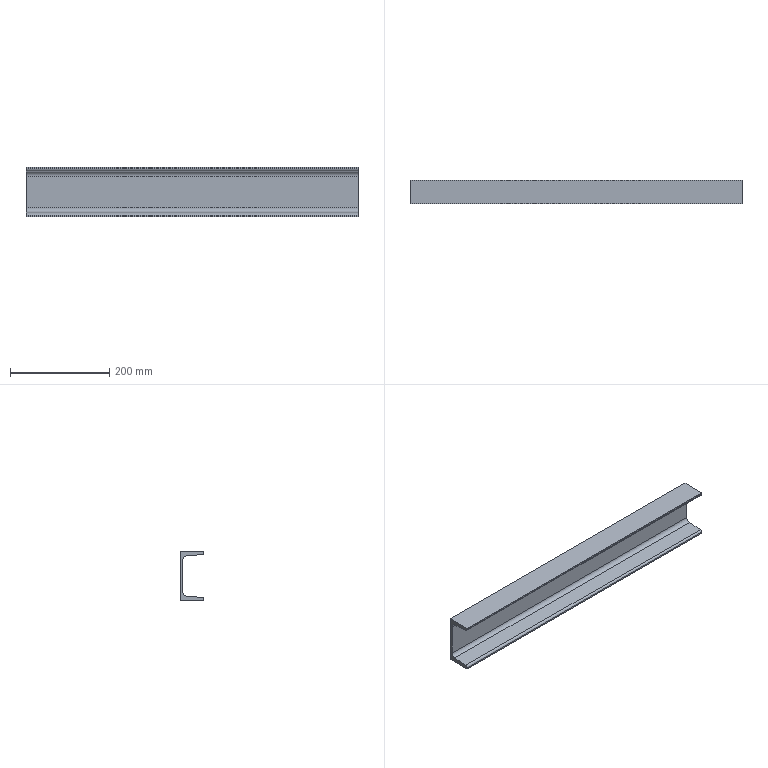Part | STEP file | 06-Channel 100x48_default<machining> | 1 solid | 14 faces | box 670 x 48 x 100 mm | volume 842936 mm3 | plane 10 | cylinder 4 | commonest cylinder face diameters 8.5 x2 17 x2
STEP:
#1=CARTESIAN_POINT('',(0.,0.,0.));
#2=DIRECTION('',(0.,0.,1.));
#3=DIRECTION('',(1.,0.,0.));
#4=AXIS2_PLACEMENT_3D('',#1,#2,#3);
#5=CARTESIAN_POINT('',(0.,-48.,-100.));
#6=VERTEX_POINT('',#5);
#7=CARTESIAN_POINT('',(0.,0.,-100.));
#8=VERTEX_POINT('',#7);
#9=CARTESIAN_POINT('',(0.,0.,-100.));
#10=DIRECTION('',(0.,1.,0.));
#11=VECTOR('',#10,1.);
#12=LINE('',#9,#11);
#13=CARTESIAN_POINT('',(670.,0.,-100.));
#14=DIRECTION('',(0.,0.,1.));
#15=DIRECTION('',(1.,0.,0.));
#16=AXIS2_PLACEMENT_3D('',#13,#14,#15);
#17=PLANE('',#16);
#18=CARTESIAN_POINT('',(-670.,0.));
#19=DIRECTION('',(0.,1.));
#20=VECTOR('',#19,1.);
#21=LINE('',#18,#20);
#22=(GEOMETRIC_REPRESENTATION_CONTEXT(2)PARAMETRIC_REPRESENTATION_CONTEXT()REPRESENTATION_CONTEXT('',''));
#23=DEFINITIONAL_REPRESENTATION('',(#21),#22);
#24=PCURVE('',#17,#23);
#25=CARTESIAN_POINT('',(0.,-43.75,-97.266));
#26=DIRECTION('',(1.,0.,0.));
#27=DIRECTION('',(0.,0.,-1.));
#28=AXIS2_PLACEMENT_3D('',#25,#26,#27);
#29=PLANE('',#28);
#30=CARTESIAN_POINT('',(2.734,43.75));
#31=DIRECTION('',(0.,1.));
#32=VECTOR('',#31,1.);
#33=LINE('',#30,#32);
#34=(GEOMETRIC_REPRESENTATION_CONTEXT(2)PARAMETRIC_REPRESENTATION_CONTEXT()REPRESENTATION_CONTEXT('',''));
#35=DEFINITIONAL_REPRESENTATION('',(#33),#34);
#36=PCURVE('',#29,#35);
#37=SURFACE_CURVE('',#12,(#24,#36),.PCURVE_S1.);
#38=EDGE_CURVE('',#6,#8,#37,.T.);
#39=ORIENTED_EDGE('',*,*,#38,.T.);
#40=CARTESIAN_POINT('',(670.,0.,-100.));
#41=VERTEX_POINT('',#40);
#42=CARTESIAN_POINT('',(670.,0.,-100.));
#43=DIRECTION('',(-1.,0.,0.));
#44=VECTOR('',#43,1.);
#45=LINE('',#42,#44);
#46=CARTESIAN_POINT('',(0.,0.));
#47=DIRECTION('',(-1.,0.));
#48=VECTOR('',#47,1.);
#49=LINE('',#46,#48);
#50=(GEOMETRIC_REPRESENTATION_CONTEXT(2)PARAMETRIC_REPRESENTATION_CONTEXT()REPRESENTATION_CONTEXT('',''));
#51=DEFINITIONAL_REPRESENTATION('',(#49),#50);
#52=PCURVE('',#17,#51);
#53=CARTESIAN_POINT('',(670.,0.,0.));
#54=DIRECTION('',(0.,-1.,0.));
#55=DIRECTION('',(0.,0.,-1.));
#56=AXIS2_PLACEMENT_3D('',#53,#54,#55);
#57=PLANE('',#56);
#58=CARTESIAN_POINT('',(100.,0.));
#59=DIRECTION('',(0.,-1.));
#60=VECTOR('',#59,1.);
#61=LINE('',#58,#60);
#62=(GEOMETRIC_REPRESENTATION_CONTEXT(2)PARAMETRIC_REPRESENTATION_CONTEXT()REPRESENTATION_CONTEXT('',''));
#63=DEFINITIONAL_REPRESENTATION('',(#61),#62);
#64=PCURVE('',#57,#63);
#65=SURFACE_CURVE('',#45,(#52,#64),.PCURVE_S1.);
#66=EDGE_CURVE('',#41,#8,#65,.T.);
#67=ORIENTED_EDGE('',*,*,#66,.F.);
#68=CARTESIAN_POINT('',(670.,-48.,-100.));
#69=VERTEX_POINT('',#68);
#70=CARTESIAN_POINT('',(670.,0.,-100.));
#71=DIRECTION('',(0.,1.,0.));
#72=VECTOR('',#71,1.);
#73=LINE('',#70,#72);
#74=CARTESIAN_POINT('',(0.,0.));
#75=DIRECTION('',(0.,1.));
#76=VECTOR('',#75,1.);
#77=LINE('',#74,#76);
#78=(GEOMETRIC_REPRESENTATION_CONTEXT(2)PARAMETRIC_REPRESENTATION_CONTEXT()REPRESENTATION_CONTEXT('',''));
#79=DEFINITIONAL_REPRESENTATION('',(#77),#78);
#80=PCURVE('',#17,#79);
#81=CARTESIAN_POINT('',(670.,-43.75,-97.266));
#82=DIRECTION('',(1.,0.,0.));
#83=DIRECTION('',(0.,0.,-1.));
#84=AXIS2_PLACEMENT_3D('',#81,#82,#83);
#85=PLANE('',#84);
#86=CARTESIAN_POINT('',(2.734,43.75));
#87=DIRECTION('',(0.,1.));
#88=VECTOR('',#87,1.);
#89=LINE('',#86,#88);
#90=(GEOMETRIC_REPRESENTATION_CONTEXT(2)PARAMETRIC_REPRESENTATION_CONTEXT()REPRESENTATION_CONTEXT('',''));
#91=DEFINITIONAL_REPRESENTATION('',(#89),#90);
#92=PCURVE('',#85,#91);
#93=SURFACE_CURVE('',#73,(#80,#92),.PCURVE_S1.);
#94=EDGE_CURVE('',#69,#41,#93,.T.);
#95=ORIENTED_EDGE('',*,*,#94,.F.);
#96=CARTESIAN_POINT('',(670.,-48.,-100.));
#97=DIRECTION('',(-1.,0.,0.));
#98=VECTOR('',#97,1.);
#99=LINE('',#96,#98);
#100=CARTESIAN_POINT('',(0.,-48.));
#101=DIRECTION('',(-1.,0.));
#102=VECTOR('',#101,1.);
#103=LINE('',#100,#102);
#104=(GEOMETRIC_REPRESENTATION_CONTEXT(2)PARAMETRIC_REPRESENTATION_CONTEXT()REPRESENTATION_CONTEXT('',''));
#105=DEFINITIONAL_REPRESENTATION('',(#103),#104);
#106=PCURVE('',#17,#105);
#107=CARTESIAN_POINT('',(670.,-48.,-97.266));
#108=DIRECTION('',(0.,1.,0.));
#109=DIRECTION('',(0.,0.,1.));
#110=AXIS2_PLACEMENT_3D('',#107,#108,#109);
#111=PLANE('',#110);
#112=CARTESIAN_POINT('',(-2.734,0.));
#113=DIRECTION('',(0.,-1.));
#114=VECTOR('',#113,1.);
#115=LINE('',#112,#114);
#116=(GEOMETRIC_REPRESENTATION_CONTEXT(2)PARAMETRIC_REPRESENTATION_CONTEXT()REPRESENTATION_CONTEXT('',''));
#117=DEFINITIONAL_REPRESENTATION('',(#115),#116);
#118=PCURVE('',#111,#117);
#119=SURFACE_CURVE('',#99,(#106,#118),.PCURVE_S1.);
#120=EDGE_CURVE('',#69,#6,#119,.T.);
#121=ORIENTED_EDGE('',*,*,#120,.T.);
#122=EDGE_LOOP('',(#39,#67,#95,#121));
#123=FACE_BOUND('',#122,.T.);
#124=ADVANCED_FACE('',(#123),#17,.F.);
#125=CARTESIAN_POINT('',(0.,0.,0.));
#126=VERTEX_POINT('',#125);
#127=CARTESIAN_POINT('',(0.,0.,0.));
#128=DIRECTION('',(0.,0.,1.));
#129=VECTOR('',#128,1.);
#130=LINE('',#127,#129);
#131=CARTESIAN_POINT('',(0.,-670.));
#132=DIRECTION('',(-1.,0.));
#133=VECTOR('',#132,1.);
#134=LINE('',#131,#133);
#135=(GEOMETRIC_REPRESENTATION_CONTEXT(2)PARAMETRIC_REPRESENTATION_CONTEXT()REPRESENTATION_CONTEXT('',''));
#136=DEFINITIONAL_REPRESENTATION('',(#134),#135);
#137=PCURVE('',#57,#136);
#138=CARTESIAN_POINT('',(-97.266,43.75));
#139=DIRECTION('',(-1.,0.));
#140=VECTOR('',#139,1.);
#141=LINE('',#138,#140);
#142=(GEOMETRIC_REPRESENTATION_CONTEXT(2)PARAMETRIC_REPRESENTATION_CONTEXT()REPRESENTATION_CONTEXT('',''));
#143=DEFINITIONAL_REPRESENTATION('',(#141),#142);
#144=PCURVE('',#29,#143);
#145=SURFACE_CURVE('',#130,(#137,#144),.PCURVE_S1.);
#146=EDGE_CURVE('',#8,#126,#145,.T.);
#147=ORIENTED_EDGE('',*,*,#146,.T.);
#148=CARTESIAN_POINT('',(670.,0.,0.));
#149=VERTEX_POINT('',#148);
#150=CARTESIAN_POINT('',(670.,0.,0.));
#151=DIRECTION('',(-1.,0.,0.));
#152=VECTOR('',#151,1.);
#153=LINE('',#150,#152);
#154=CARTESIAN_POINT('',(0.,0.));
#155=DIRECTION('',(0.,-1.));
#156=VECTOR('',#155,1.);
#157=LINE('',#154,#156);
#158=(GEOMETRIC_REPRESENTATION_CONTEXT(2)PARAMETRIC_REPRESENTATION_CONTEXT()REPRESENTATION_CONTEXT('',''));
#159=DEFINITIONAL_REPRESENTATION('',(#157),#158);
#160=PCURVE('',#57,#159);
#161=CARTESIAN_POINT('',(670.,0.,0.));
#162=DIRECTION('',(0.,0.,-1.));
#163=DIRECTION('',(0.,1.,0.));
#164=AXIS2_PLACEMENT_3D('',#161,#162,#163);
#165=PLANE('',#164);
#166=CARTESIAN_POINT('',(0.,0.));
#167=DIRECTION('',(0.,-1.));
#168=VECTOR('',#167,1.);
#169=LINE('',#166,#168);
#170=(GEOMETRIC_REPRESENTATION_CONTEXT(2)PARAMETRIC_REPRESENTATION_CONTEXT()REPRESENTATION_CONTEXT('',''));
#171=DEFINITIONAL_REPRESENTATION('',(#169),#170);
#172=PCURVE('',#165,#171);
#173=SURFACE_CURVE('',#153,(#160,#172),.PCURVE_S1.);
#174=EDGE_CURVE('',#149,#126,#173,.T.);
#175=ORIENTED_EDGE('',*,*,#174,.F.);
#176=CARTESIAN_POINT('',(670.,0.,0.));
#177=DIRECTION('',(0.,0.,1.));
#178=VECTOR('',#177,1.);
#179=LINE('',#176,#178);
#180=CARTESIAN_POINT('',(0.,0.));
#181=DIRECTION('',(-1.,0.));
#182=VECTOR('',#181,1.);
#183=LINE('',#180,#182);
#184=(GEOMETRIC_REPRESENTATION_CONTEXT(2)PARAMETRIC_REPRESENTATION_CONTEXT()REPRESENTATION_CONTEXT('',''));
#185=DEFINITIONAL_REPRESENTATION('',(#183),#184);
#186=PCURVE('',#57,#185);
#187=CARTESIAN_POINT('',(-97.266,43.75));
#188=DIRECTION('',(-1.,0.));
#189=VECTOR('',#188,1.);
#190=LINE('',#187,#189);
#191=(GEOMETRIC_REPRESENTATION_CONTEXT(2)PARAMETRIC_REPRESENTATION_CONTEXT()REPRESENTATION_CONTEXT('',''));
#192=DEFINITIONAL_REPRESENTATION('',(#190),#191);
#193=PCURVE('',#85,#192);
#194=SURFACE_CURVE('',#179,(#186,#193),.PCURVE_S1.);
#195=EDGE_CURVE('',#41,#149,#194,.T.);
#196=ORIENTED_EDGE('',*,*,#195,.F.);
#197=ORIENTED_EDGE('',*,*,#66,.T.);
#198=EDGE_LOOP('',(#147,#175,#196,#197));
#199=FACE_BOUND('',#198,.T.);
#200=ADVANCED_FACE('',(#199),#57,.F.);
#201=CARTESIAN_POINT('',(0.,-48.,0.));
#202=VERTEX_POINT('',#201);
#203=CARTESIAN_POINT('',(0.,0.,0.));
#204=DIRECTION('',(0.,-1.,0.));
#205=VECTOR('',#204,1.);
#206=LINE('',#203,#205);
#207=CARTESIAN_POINT('',(0.,-670.));
#208=DIRECTION('',(-1.,0.));
#209=VECTOR('',#208,1.);
#210=LINE('',#207,#209);
#211=(GEOMETRIC_REPRESENTATION_CONTEXT(2)PARAMETRIC_REPRESENTATION_CONTEXT()REPRESENTATION_CONTEXT('',''));
#212=DEFINITIONAL_REPRESENTATION('',(#210),#211);
#213=PCURVE('',#165,#212);
#214=CARTESIAN_POINT('',(-97.266,43.75));
#215=DIRECTION('',(0.,-1.));
#216=VECTOR('',#215,1.);
#217=LINE('',#214,#216);
#218=(GEOMETRIC_REPRESENTATION_CONTEXT(2)PARAMETRIC_REPRESENTATION_CONTEXT()REPRESENTATION_CONTEXT('',''));
#219=DEFINITIONAL_REPRESENTATION('',(#217),#218);
#220=PCURVE('',#29,#219);
#221=SURFACE_CURVE('',#206,(#213,#220),.PCURVE_S1.);
#222=EDGE_CURVE('',#126,#202,#221,.T.);
#223=ORIENTED_EDGE('',*,*,#222,.T.);
#224=CARTESIAN_POINT('',(670.,-48.,0.));
#225=VERTEX_POINT('',#224);
#226=CARTESIAN_POINT('',(670.,-48.,0.));
#227=DIRECTION('',(-1.,0.,0.));
#228=VECTOR('',#227,1.);
#229=LINE('',#226,#228);
#230=CARTESIAN_POINT('',(-48.,0.));
#231=DIRECTION('',(0.,-1.));
#232=VECTOR('',#231,1.);
#233=LINE('',#230,#232);
#234=(GEOMETRIC_REPRESENTATION_CONTEXT(2)PARAMETRIC_REPRESENTATION_CONTEXT()REPRESENTATION_CONTEXT('',''));
#235=DEFINITIONAL_REPRESENTATION('',(#233),#234);
#236=PCURVE('',#165,#235);
#237=CARTESIAN_POINT('',(670.,-48.,-2.734));
#238=DIRECTION('',(0.,1.,0.));
#239=DIRECTION('',(0.,0.,1.));
#240=AXIS2_PLACEMENT_3D('',#237,#238,#239);
#241=PLANE('',#240);
#242=CARTESIAN_POINT('',(2.734,0.));
#243=DIRECTION('',(0.,-1.));
#244=VECTOR('',#243,1.);
#245=LINE('',#242,#244);
#246=(GEOMETRIC_REPRESENTATION_CONTEXT(2)PARAMETRIC_REPRESENTATION_CONTEXT()REPRESENTATION_CONTEXT('',''));
#247=DEFINITIONAL_REPRESENTATION('',(#245),#246);
#248=PCURVE('',#241,#247);
#249=SURFACE_CURVE('',#229,(#236,#248),.PCURVE_S1.);
#250=EDGE_CURVE('',#225,#202,#249,.T.);
#251=ORIENTED_EDGE('',*,*,#250,.F.);
#252=CARTESIAN_POINT('',(670.,0.,0.));
#253=DIRECTION('',(0.,-1.,0.));
#254=VECTOR('',#253,1.);
#255=LINE('',#252,#254);
#256=CARTESIAN_POINT('',(0.,0.));
#257=DIRECTION('',(-1.,0.));
#258=VECTOR('',#257,1.);
#259=LINE('',#256,#258);
#260=(GEOMETRIC_REPRESENTATION_CONTEXT(2)PARAMETRIC_REPRESENTATION_CONTEXT()REPRESENTATION_CONTEXT('',''));
#261=DEFINITIONAL_REPRESENTATION('',(#259),#260);
#262=PCURVE('',#165,#261);
#263=CARTESIAN_POINT('',(-97.266,43.75));
#264=DIRECTION('',(0.,-1.));
#265=VECTOR('',#264,1.);
#266=LINE('',#263,#265);
#267=(GEOMETRIC_REPRESENTATION_CONTEXT(2)PARAMETRIC_REPRESENTATION_CONTEXT()REPRESENTATION_CONTEXT('',''));
#268=DEFINITIONAL_REPRESENTATION('',(#266),#267);
#269=PCURVE('',#85,#268);
#270=SURFACE_CURVE('',#255,(#262,#269),.PCURVE_S1.);
#271=EDGE_CURVE('',#149,#225,#270,.T.);
#272=ORIENTED_EDGE('',*,*,#271,.F.);
#273=ORIENTED_EDGE('',*,*,#174,.T.);
#274=EDGE_LOOP('',(#223,#251,#272,#273));
#275=FACE_BOUND('',#274,.T.);
#276=ADVANCED_FACE('',(#275),#165,.F.);
#277=CARTESIAN_POINT('',(0.,-48.,-2.734));
#278=VERTEX_POINT('',#277);
#279=CARTESIAN_POINT('',(0.,-48.,-2.734));
#280=DIRECTION('',(0.,0.,-1.));
#281=VECTOR('',#280,1.);
#282=LINE('',#279,#281);
#283=CARTESIAN_POINT('',(0.,-670.));
#284=DIRECTION('',(-1.,0.));
#285=VECTOR('',#284,1.);
#286=LINE('',#283,#285);
#287=(GEOMETRIC_REPRESENTATION_CONTEXT(2)PARAMETRIC_REPRESENTATION_CONTEXT()REPRESENTATION_CONTEXT('',''));
#288=DEFINITIONAL_REPRESENTATION('',(#286),#287);
#289=PCURVE('',#241,#288);
#290=CARTESIAN_POINT('',(-94.531,-4.25));
#291=DIRECTION('',(1.,0.));
#292=VECTOR('',#291,1.);
#293=LINE('',#290,#292);
#294=(GEOMETRIC_REPRESENTATION_CONTEXT(2)PARAMETRIC_REPRESENTATION_CONTEXT()REPRESENTATION_CONTEXT('',''));
#295=DEFINITIONAL_REPRESENTATION('',(#293),#294);
#296=PCURVE('',#29,#295);
#297=SURFACE_CURVE('',#282,(#289,#296),.PCURVE_S1.);
#298=EDGE_CURVE('',#202,#278,#297,.T.);
#299=ORIENTED_EDGE('',*,*,#298,.T.);
#300=CARTESIAN_POINT('',(670.,-48.,-2.734));
#301=VERTEX_POINT('',#300);
#302=CARTESIAN_POINT('',(670.,-48.,-2.734));
#303=DIRECTION('',(-1.,0.,0.));
#304=VECTOR('',#303,1.);
#305=LINE('',#302,#304);
#306=CARTESIAN_POINT('',(0.,0.));
#307=DIRECTION('',(0.,-1.));
#308=VECTOR('',#307,1.);
#309=LINE('',#306,#308);
#310=(GEOMETRIC_REPRESENTATION_CONTEXT(2)PARAMETRIC_REPRESENTATION_CONTEXT()REPRESENTATION_CONTEXT('',''));
#311=DEFINITIONAL_REPRESENTATION('',(#309),#310);
#312=PCURVE('',#241,#311);
#313=CARTESIAN_POINT('',(670.,-43.75,-2.734));
#314=DIRECTION('',(-1.,0.,0.));
#315=DIRECTION('',(0.,0.,1.));
#316=AXIS2_PLACEMENT_3D('',#313,#314,#315);
#317=CYLINDRICAL_SURFACE('',#316,4.25);
#318=CARTESIAN_POINT('',(4.712,0.));
#319=DIRECTION('',(0.,1.));
#320=VECTOR('',#319,1.);
#321=LINE('',#318,#320);
#322=(GEOMETRIC_REPRESENTATION_CONTEXT(2)PARAMETRIC_REPRESENTATION_CONTEXT()REPRESENTATION_CONTEXT('',''));
#323=DEFINITIONAL_REPRESENTATION('',(#321),#322);
#324=PCURVE('',#317,#323);
#325=SURFACE_CURVE('',#305,(#312,#324),.PCURVE_S1.);
#326=EDGE_CURVE('',#301,#278,#325,.T.);
#327=ORIENTED_EDGE('',*,*,#326,.F.);
#328=CARTESIAN_POINT('',(670.,-48.,-2.734));
#329=DIRECTION('',(0.,0.,-1.));
#330=VECTOR('',#329,1.);
#331=LINE('',#328,#330);
#332=CARTESIAN_POINT('',(0.,0.));
#333=DIRECTION('',(-1.,0.));
#334=VECTOR('',#333,1.);
#335=LINE('',#332,#334);
#336=(GEOMETRIC_REPRESENTATION_CONTEXT(2)PARAMETRIC_REPRESENTATION_CONTEXT()REPRESENTATION_CONTEXT('',''));
#337=DEFINITIONAL_REPRESENTATION('',(#335),#336);
#338=PCURVE('',#241,#337);
#339=CARTESIAN_POINT('',(-94.531,-4.25));
#340=DIRECTION('',(1.,0.));
#341=VECTOR('',#340,1.);
#342=LINE('',#339,#341);
#343=(GEOMETRIC_REPRESENTATION_CONTEXT(2)PARAMETRIC_REPRESENTATION_CONTEXT()REPRESENTATION_CONTEXT('',''));
#344=DEFINITIONAL_REPRESENTATION('',(#342),#343);
#345=PCURVE('',#85,#344);
#346=SURFACE_CURVE('',#331,(#338,#345),.PCURVE_S1.);
#347=EDGE_CURVE('',#225,#301,#346,.T.);
#348=ORIENTED_EDGE('',*,*,#347,.F.);
#349=ORIENTED_EDGE('',*,*,#250,.T.);
#350=EDGE_LOOP('',(#299,#327,#348,#349));
#351=FACE_BOUND('',#350,.T.);
#352=ADVANCED_FACE('',(#351),#241,.F.);
#353=CARTESIAN_POINT('',(0.,-44.073,-6.972));
#354=VERTEX_POINT('',#353);
#355=CARTESIAN_POINT('',(0.,-43.75,-2.734));
#356=DIRECTION('',(1.,0.,0.));
#357=DIRECTION('',(0.,0.,-1.));
#358=AXIS2_PLACEMENT_3D('',#355,#356,#357);
#359=CIRCLE('',#358,4.25);
#360=CARTESIAN_POINT('',(9.425,670.));
#361=DIRECTION('',(-1.,0.));
#362=VECTOR('',#361,1.);
#363=LINE('',#360,#362);
#364=(GEOMETRIC_REPRESENTATION_CONTEXT(2)PARAMETRIC_REPRESENTATION_CONTEXT()REPRESENTATION_CONTEXT('',''));
#365=DEFINITIONAL_REPRESENTATION('',(#363),#364);
#366=PCURVE('',#317,#365);
#367=CARTESIAN_POINT('',(-94.531,0.));
#368=DIRECTION('',(1.,0.));
#369=AXIS2_PLACEMENT_2D('',#367,#368);
#370=CIRCLE('',#369,4.25);
#371=(GEOMETRIC_REPRESENTATION_CONTEXT(2)PARAMETRIC_REPRESENTATION_CONTEXT()REPRESENTATION_CONTEXT('',''));
#372=DEFINITIONAL_REPRESENTATION('',(#370),#371);
#373=PCURVE('',#29,#372);
#374=SURFACE_CURVE('',#359,(#366,#373),.PCURVE_S1.);
#375=EDGE_CURVE('',#278,#354,#374,.T.);
#376=ORIENTED_EDGE('',*,*,#375,.T.);
#377=CARTESIAN_POINT('',(670.,-44.073,-6.972));
#378=VERTEX_POINT('',#377);
#379=CARTESIAN_POINT('',(670.,-44.073,-6.972));
#380=DIRECTION('',(-1.,0.,0.));
#381=VECTOR('',#380,1.);
#382=LINE('',#379,#381);
#383=CARTESIAN_POINT('',(3.218,0.));
#384=DIRECTION('',(0.,1.));
#385=VECTOR('',#384,1.);
#386=LINE('',#383,#385);
#387=(GEOMETRIC_REPRESENTATION_CONTEXT(2)PARAMETRIC_REPRESENTATION_CONTEXT()REPRESENTATION_CONTEXT('',''));
#388=DEFINITIONAL_REPRESENTATION('',(#386),#387);
#389=PCURVE('',#317,#388);
#390=CARTESIAN_POINT('',(670.,-13.155,-9.325));
#391=DIRECTION('',(0.,0.07589,0.9971));
#392=DIRECTION('',(0.,-0.9971,0.07589));
#393=AXIS2_PLACEMENT_3D('',#390,#391,#392);
#394=PLANE('',#393);
#395=CARTESIAN_POINT('',(31.007,0.));
#396=DIRECTION('',(0.,-1.));
#397=VECTOR('',#396,1.);
#398=LINE('',#395,#397);
#399=(GEOMETRIC_REPRESENTATION_CONTEXT(2)PARAMETRIC_REPRESENTATION_CONTEXT()REPRESENTATION_CONTEXT('',''));
#400=DEFINITIONAL_REPRESENTATION('',(#398),#399);
#401=PCURVE('',#394,#400);
#402=SURFACE_CURVE('',#382,(#389,#401),.PCURVE_S1.);
#403=EDGE_CURVE('',#378,#354,#402,.T.);
#404=ORIENTED_EDGE('',*,*,#403,.F.);
#405=CARTESIAN_POINT('',(670.,-43.75,-2.734));
#406=DIRECTION('',(1.,0.,0.));
#407=DIRECTION('',(0.,0.,-1.));
#408=AXIS2_PLACEMENT_3D('',#405,#406,#407);
#409=CIRCLE('',#408,4.25);
#410=CARTESIAN_POINT('',(9.425,0.));
#411=DIRECTION('',(-1.,0.));
#412=VECTOR('',#411,1.);
#413=LINE('',#410,#412);
#414=(GEOMETRIC_REPRESENTATION_CONTEXT(2)PARAMETRIC_REPRESENTATION_CONTEXT()REPRESENTATION_CONTEXT('',''));
#415=DEFINITIONAL_REPRESENTATION('',(#413),#414);
#416=PCURVE('',#317,#415);
#417=CARTESIAN_POINT('',(-94.531,0.));
#418=DIRECTION('',(1.,0.));
#419=AXIS2_PLACEMENT_2D('',#417,#418);
#420=CIRCLE('',#419,4.25);
#421=(GEOMETRIC_REPRESENTATION_CONTEXT(2)PARAMETRIC_REPRESENTATION_CONTEXT()REPRESENTATION_CONTEXT('',''));
#422=DEFINITIONAL_REPRESENTATION('',(#420),#421);
#423=PCURVE('',#85,#422);
#424=SURFACE_CURVE('',#409,(#416,#423),.PCURVE_S1.);
#425=EDGE_CURVE('',#301,#378,#424,.T.);
#426=ORIENTED_EDGE('',*,*,#425,.F.);
#427=ORIENTED_EDGE('',*,*,#326,.T.);
#428=EDGE_LOOP('',(#376,#404,#426,#427));
#429=FACE_BOUND('',#428,.T.);
#430=ADVANCED_FACE('',(#429),#317,.T.);
#431=CARTESIAN_POINT('',(0.,-13.155,-9.325));
#432=VERTEX_POINT('',#431);
#433=CARTESIAN_POINT('',(0.,-13.155,-9.325));
#434=DIRECTION('',(0.,0.9971,-0.07589));
#435=VECTOR('',#434,1.);
#436=LINE('',#433,#435);
#437=CARTESIAN_POINT('',(0.,-670.));
#438=DIRECTION('',(-1.,0.));
#439=VECTOR('',#438,1.);
#440=LINE('',#437,#439);
#441=(GEOMETRIC_REPRESENTATION_CONTEXT(2)PARAMETRIC_REPRESENTATION_CONTEXT()REPRESENTATION_CONTEXT('',''));
#442=DEFINITIONAL_REPRESENTATION('',(#440),#441);
#443=PCURVE('',#394,#442);
#444=CARTESIAN_POINT('',(-87.94,30.595));
#445=DIRECTION('',(0.07589,0.9971));
#446=VECTOR('',#445,1.);
#447=LINE('',#444,#446);
#448=(GEOMETRIC_REPRESENTATION_CONTEXT(2)PARAMETRIC_REPRESENTATION_CONTEXT()REPRESENTATION_CONTEXT('',''));
#449=DEFINITIONAL_REPRESENTATION('',(#447),#448);
#450=PCURVE('',#29,#449);
#451=SURFACE_CURVE('',#436,(#443,#450),.PCURVE_S1.);
#452=EDGE_CURVE('',#354,#432,#451,.T.);
#453=ORIENTED_EDGE('',*,*,#452,.T.);
#454=CARTESIAN_POINT('',(670.,-13.155,-9.325));
#455=VERTEX_POINT('',#454);
#456=CARTESIAN_POINT('',(670.,-13.155,-9.325));
#457=DIRECTION('',(-1.,0.,0.));
#458=VECTOR('',#457,1.);
#459=LINE('',#456,#458);
#460=CARTESIAN_POINT('',(0.,0.));
#461=DIRECTION('',(0.,-1.));
#462=VECTOR('',#461,1.);
#463=LINE('',#460,#462);
#464=(GEOMETRIC_REPRESENTATION_CONTEXT(2)PARAMETRIC_REPRESENTATION_CONTEXT()REPRESENTATION_CONTEXT('',''));
#465=DEFINITIONAL_REPRESENTATION('',(#463),#464);
#466=PCURVE('',#394,#465);
#467=CARTESIAN_POINT('',(670.,-13.8,-17.801));
#468=DIRECTION('',(-1.,0.,0.));
#469=DIRECTION('',(0.,0.,1.));
#470=AXIS2_PLACEMENT_3D('',#467,#468,#469);
#471=CYLINDRICAL_SURFACE('',#470,8.5);
#472=CARTESIAN_POINT('',(0.07597,0.));
#473=DIRECTION('',(0.,1.));
#474=VECTOR('',#473,1.);
#475=LINE('',#472,#474);
#476=(GEOMETRIC_REPRESENTATION_CONTEXT(2)PARAMETRIC_REPRESENTATION_CONTEXT()REPRESENTATION_CONTEXT('',''));
#477=DEFINITIONAL_REPRESENTATION('',(#475),#476);
#478=PCURVE('',#471,#477);
#479=SURFACE_CURVE('',#459,(#466,#478),.PCURVE_S1.);
#480=EDGE_CURVE('',#455,#432,#479,.T.);
#481=ORIENTED_EDGE('',*,*,#480,.F.);
#482=CARTESIAN_POINT('',(670.,-13.155,-9.325));
#483=DIRECTION('',(0.,0.9971,-0.07589));
#484=VECTOR('',#483,1.);
#485=LINE('',#482,#484);
#486=CARTESIAN_POINT('',(0.,0.));
#487=DIRECTION('',(-1.,0.));
#488=VECTOR('',#487,1.);
#489=LINE('',#486,#488);
#490=(GEOMETRIC_REPRESENTATION_CONTEXT(2)PARAMETRIC_REPRESENTATION_CONTEXT()REPRESENTATION_CONTEXT('',''));
#491=DEFINITIONAL_REPRESENTATION('',(#489),#490);
#492=PCURVE('',#394,#491);
#493=CARTESIAN_POINT('',(-87.94,30.595));
#494=DIRECTION('',(0.07589,0.9971));
#495=VECTOR('',#494,1.);
#496=LINE('',#493,#495);
#497=(GEOMETRIC_REPRESENTATION_CONTEXT(2)PARAMETRIC_REPRESENTATION_CONTEXT()REPRESENTATION_CONTEXT('',''));
#498=DEFINITIONAL_REPRESENTATION('',(#496),#497);
#499=PCURVE('',#85,#498);
#500=SURFACE_CURVE('',#485,(#492,#499),.PCURVE_S1.);
#501=EDGE_CURVE('',#378,#455,#500,.T.);
#502=ORIENTED_EDGE('',*,*,#501,.F.);
#503=ORIENTED_EDGE('',*,*,#403,.T.);
#504=EDGE_LOOP('',(#453,#481,#502,#503));
#505=FACE_BOUND('',#504,.T.);
#506=ADVANCED_FACE('',(#505),#394,.F.);
#507=ORIENTED_EDGE('',*,*,#480,.F.);
#508=CARTESIAN_POINT('',(670.,-5.3,-17.801));
#509=VERTEX_POINT('',#508);
#510=CARTESIAN_POINT('',(670.,-13.8,-17.801));
#511=DIRECTION('',(-1.,0.,0.));
#512=DIRECTION('',(0.,0.,1.));
#513=AXIS2_PLACEMENT_3D('',#510,#511,#512);
#514=CIRCLE('',#513,8.5);
#515=CARTESIAN_POINT('',(0.,0.));
#516=DIRECTION('',(1.,0.));
#517=VECTOR('',#516,1.);
#518=LINE('',#515,#517);
#519=(GEOMETRIC_REPRESENTATION_CONTEXT(2)PARAMETRIC_REPRESENTATION_CONTEXT()REPRESENTATION_CONTEXT('',''));
#520=DEFINITIONAL_REPRESENTATION('',(#518),#519);
#521=PCURVE('',#471,#520);
#522=CARTESIAN_POINT('',(-87.965,29.95));
#523=CARTESIAN_POINT('',(-87.965,44.672));
#524=CARTESIAN_POINT('',(-75.215,37.311));
#525=CARTESIAN_POINT('',(-62.465,29.95));
#526=CARTESIAN_POINT('',(-75.215,22.589));
#527=CARTESIAN_POINT('',(-87.965,15.228));
#528=CARTESIAN_POINT('',(-87.965,29.95));
#529=(BOUNDED_CURVE()B_SPLINE_CURVE(2,(#522,#523,#524,#525,#526,#527,#528),.UNSPECIFIED.,.T.,.F.)B_SPLINE_CURVE_WITH_KNOTS((1,2,2,2,2,1),(-2.094,0.,2.094,4.189,6.283,8.378),.UNSPECIFIED.)CURVE()GEOMETRIC_REPRESENTATION_ITEM()RATIONAL_B_SPLINE_CURVE((1.,0.5,1.,0.5,1.,0.5,1.))REPRESENTATION_ITEM(''));
#530=(GEOMETRIC_REPRESENTATION_CONTEXT(2)PARAMETRIC_REPRESENTATION_CONTEXT()REPRESENTATION_CONTEXT('',''));
#531=DEFINITIONAL_REPRESENTATION('',(#529),#530);
#532=PCURVE('',#85,#531);
#533=SURFACE_CURVE('',#514,(#521,#532),.PCURVE_S1.);
#534=EDGE_CURVE('',#455,#509,#533,.T.);
#535=ORIENTED_EDGE('',*,*,#534,.T.);
#536=CARTESIAN_POINT('',(0.,-5.3,-17.801));
#537=VERTEX_POINT('',#536);
#538=CARTESIAN_POINT('',(670.,-5.3,-17.801));
#539=DIRECTION('',(-1.,0.,0.));
#540=VECTOR('',#539,1.);
#541=LINE('',#538,#540);
#542=CARTESIAN_POINT('',(1.571,0.));
#543=DIRECTION('',(0.,1.));
#544=VECTOR('',#543,1.);
#545=LINE('',#542,#544);
#546=(GEOMETRIC_REPRESENTATION_CONTEXT(2)PARAMETRIC_REPRESENTATION_CONTEXT()REPRESENTATION_CONTEXT('',''));
#547=DEFINITIONAL_REPRESENTATION('',(#545),#546);
#548=PCURVE('',#471,#547);
#549=CARTESIAN_POINT('',(670.,-5.3,-82.199));
#550=DIRECTION('',(0.,1.,0.));
#551=DIRECTION('',(0.,0.,1.));
#552=AXIS2_PLACEMENT_3D('',#549,#550,#551);
#553=PLANE('',#552);
#554=CARTESIAN_POINT('',(64.398,0.));
#555=DIRECTION('',(0.,-1.));
#556=VECTOR('',#555,1.);
#557=LINE('',#554,#556);
#558=(GEOMETRIC_REPRESENTATION_CONTEXT(2)PARAMETRIC_REPRESENTATION_CONTEXT()REPRESENTATION_CONTEXT('',''));
#559=DEFINITIONAL_REPRESENTATION('',(#557),#558);
#560=PCURVE('',#553,#559);
#561=SURFACE_CURVE('',#541,(#548,#560),.PCURVE_S1.);
#562=EDGE_CURVE('',#509,#537,#561,.T.);
#563=ORIENTED_EDGE('',*,*,#562,.T.);
#564=CARTESIAN_POINT('',(0.,-13.8,-17.801));
#565=DIRECTION('',(-1.,0.,0.));
#566=DIRECTION('',(0.,0.,1.));
#567=AXIS2_PLACEMENT_3D('',#564,#565,#566);
#568=CIRCLE('',#567,8.5);
#569=CARTESIAN_POINT('',(0.,670.));
#570=DIRECTION('',(1.,0.));
#571=VECTOR('',#570,1.);
#572=LINE('',#569,#571);
#573=(GEOMETRIC_REPRESENTATION_CONTEXT(2)PARAMETRIC_REPRESENTATION_CONTEXT()REPRESENTATION_CONTEXT('',''));
#574=DEFINITIONAL_REPRESENTATION('',(#572),#573);
#575=PCURVE('',#471,#574);
#576=CARTESIAN_POINT('',(-87.965,29.95));
#577=CARTESIAN_POINT('',(-87.965,44.672));
#578=CARTESIAN_POINT('',(-75.215,37.311));
#579=CARTESIAN_POINT('',(-62.465,29.95));
#580=CARTESIAN_POINT('',(-75.215,22.589));
#581=CARTESIAN_POINT('',(-87.965,15.228));
#582=CARTESIAN_POINT('',(-87.965,29.95));
#583=(BOUNDED_CURVE()B_SPLINE_CURVE(2,(#576,#577,#578,#579,#580,#581,#582),.UNSPECIFIED.,.T.,.F.)B_SPLINE_CURVE_WITH_KNOTS((1,2,2,2,2,1),(-2.094,0.,2.094,4.189,6.283,8.378),.UNSPECIFIED.)CURVE()GEOMETRIC_REPRESENTATION_ITEM()RATIONAL_B_SPLINE_CURVE((1.,0.5,1.,0.5,1.,0.5,1.))REPRESENTATION_ITEM(''));
#584=(GEOMETRIC_REPRESENTATION_CONTEXT(2)PARAMETRIC_REPRESENTATION_CONTEXT()REPRESENTATION_CONTEXT('',''));
#585=DEFINITIONAL_REPRESENTATION('',(#583),#584);
#586=PCURVE('',#29,#585);
#587=SURFACE_CURVE('',#568,(#575,#586),.PCURVE_S1.);
#588=EDGE_CURVE('',#432,#537,#587,.T.);
#589=ORIENTED_EDGE('',*,*,#588,.F.);
#590=EDGE_LOOP('',(#507,#535,#563,#589));
#591=FACE_BOUND('',#590,.F.);
#592=ADVANCED_FACE('',(#591),#471,.F.);
#593=CARTESIAN_POINT('',(0.,-5.3,-82.199));
#594=VERTEX_POINT('',#593);
#595=CARTESIAN_POINT('',(0.,-5.3,-82.199));
#596=DIRECTION('',(0.,0.,-1.));
#597=VECTOR('',#596,1.);
#598=LINE('',#595,#597);
#599=CARTESIAN_POINT('',(0.,-670.));
#600=DIRECTION('',(-1.,0.));
#601=VECTOR('',#600,1.);
#602=LINE('',#599,#601);
#603=(GEOMETRIC_REPRESENTATION_CONTEXT(2)PARAMETRIC_REPRESENTATION_CONTEXT()REPRESENTATION_CONTEXT('',''));
#604=DEFINITIONAL_REPRESENTATION('',(#602),#603);
#605=PCURVE('',#553,#604);
#606=CARTESIAN_POINT('',(-15.066,38.45));
#607=DIRECTION('',(1.,0.));
#608=VECTOR('',#607,1.);
#609=LINE('',#606,#608);
#610=(GEOMETRIC_REPRESENTATION_CONTEXT(2)PARAMETRIC_REPRESENTATION_CONTEXT()REPRESENTATION_CONTEXT('',''));
#611=DEFINITIONAL_REPRESENTATION('',(#609),#610);
#612=PCURVE('',#29,#611);
#613=SURFACE_CURVE('',#598,(#605,#612),.PCURVE_S1.);
#614=EDGE_CURVE('',#537,#594,#613,.T.);
#615=ORIENTED_EDGE('',*,*,#614,.T.);
#616=CARTESIAN_POINT('',(670.,-5.3,-82.199));
#617=VERTEX_POINT('',#616);
#618=CARTESIAN_POINT('',(670.,-5.3,-82.199));
#619=DIRECTION('',(-1.,0.,0.));
#620=VECTOR('',#619,1.);
#621=LINE('',#618,#620);
#622=CARTESIAN_POINT('',(0.,0.));
#623=DIRECTION('',(0.,-1.));
#624=VECTOR('',#623,1.);
#625=LINE('',#622,#624);
#626=(GEOMETRIC_REPRESENTATION_CONTEXT(2)PARAMETRIC_REPRESENTATION_CONTEXT()REPRESENTATION_CONTEXT('',''));
#627=DEFINITIONAL_REPRESENTATION('',(#625),#626);
#628=PCURVE('',#553,#627);
#629=CARTESIAN_POINT('',(670.,-13.8,-82.199));
#630=DIRECTION('',(-1.,0.,0.));
#631=DIRECTION('',(0.,0.,1.));
#632=AXIS2_PLACEMENT_3D('',#629,#630,#631);
#633=CYLINDRICAL_SURFACE('',#632,8.5);
#634=CARTESIAN_POINT('',(1.571,0.));
#635=DIRECTION('',(0.,1.));
#636=VECTOR('',#635,1.);
#637=LINE('',#634,#636);
#638=(GEOMETRIC_REPRESENTATION_CONTEXT(2)PARAMETRIC_REPRESENTATION_CONTEXT()REPRESENTATION_CONTEXT('',''));
#639=DEFINITIONAL_REPRESENTATION('',(#637),#638);
#640=PCURVE('',#633,#639);
#641=SURFACE_CURVE('',#621,(#628,#640),.PCURVE_S1.);
#642=EDGE_CURVE('',#617,#594,#641,.T.);
#643=ORIENTED_EDGE('',*,*,#642,.F.);
#644=CARTESIAN_POINT('',(670.,-5.3,-82.199));
#645=DIRECTION('',(0.,0.,-1.));
#646=VECTOR('',#645,1.);
#647=LINE('',#644,#646);
#648=CARTESIAN_POINT('',(0.,0.));
#649=DIRECTION('',(-1.,0.));
#650=VECTOR('',#649,1.);
#651=LINE('',#648,#650);
#652=(GEOMETRIC_REPRESENTATION_CONTEXT(2)PARAMETRIC_REPRESENTATION_CONTEXT()REPRESENTATION_CONTEXT('',''));
#653=DEFINITIONAL_REPRESENTATION('',(#651),#652);
#654=PCURVE('',#553,#653);
#655=CARTESIAN_POINT('',(-15.066,38.45));
#656=DIRECTION('',(1.,0.));
#657=VECTOR('',#656,1.);
#658=LINE('',#655,#657);
#659=(GEOMETRIC_REPRESENTATION_CONTEXT(2)PARAMETRIC_REPRESENTATION_CONTEXT()REPRESENTATION_CONTEXT('',''));
#660=DEFINITIONAL_REPRESENTATION('',(#658),#659);
#661=PCURVE('',#85,#660);
#662=SURFACE_CURVE('',#647,(#654,#661),.PCURVE_S1.);
#663=EDGE_CURVE('',#509,#617,#662,.T.);
#664=ORIENTED_EDGE('',*,*,#663,.F.);
#665=ORIENTED_EDGE('',*,*,#562,.T.);
#666=EDGE_LOOP('',(#615,#643,#664,#665));
#667=FACE_BOUND('',#666,.T.);
#668=ADVANCED_FACE('',(#667),#553,.F.);
#669=ORIENTED_EDGE('',*,*,#642,.F.);
#670=CARTESIAN_POINT('',(670.,-13.155,-90.675));
#671=VERTEX_POINT('',#670);
#672=CARTESIAN_POINT('',(670.,-13.8,-82.199));
#673=DIRECTION('',(-1.,0.,0.));
#674=DIRECTION('',(0.,0.,1.));
#675=AXIS2_PLACEMENT_3D('',#672,#673,#674);
#676=CIRCLE('',#675,8.5);
#677=CARTESIAN_POINT('',(0.,0.));
#678=DIRECTION('',(1.,0.));
#679=VECTOR('',#678,1.);
#680=LINE('',#677,#679);
#681=(GEOMETRIC_REPRESENTATION_CONTEXT(2)PARAMETRIC_REPRESENTATION_CONTEXT()REPRESENTATION_CONTEXT('',''));
#682=DEFINITIONAL_REPRESENTATION('',(#680),#681);
#683=PCURVE('',#633,#682);
#684=CARTESIAN_POINT('',(-23.566,29.95));
#685=CARTESIAN_POINT('',(-23.566,44.672));
#686=CARTESIAN_POINT('',(-10.816,37.311));
#687=CARTESIAN_POINT('',(1.934,29.95));
#688=CARTESIAN_POINT('',(-10.816,22.589));
#689=CARTESIAN_POINT('',(-23.566,15.228));
#690=CARTESIAN_POINT('',(-23.566,29.95));
#691=(BOUNDED_CURVE()B_SPLINE_CURVE(2,(#684,#685,#686,#687,#688,#689,#690),.UNSPECIFIED.,.T.,.F.)B_SPLINE_CURVE_WITH_KNOTS((1,2,2,2,2,1),(-2.094,0.,2.094,4.189,6.283,8.378),.UNSPECIFIED.)CURVE()GEOMETRIC_REPRESENTATION_ITEM()RATIONAL_B_SPLINE_CURVE((1.,0.5,1.,0.5,1.,0.5,1.))REPRESENTATION_ITEM(''));
#692=(GEOMETRIC_REPRESENTATION_CONTEXT(2)PARAMETRIC_REPRESENTATION_CONTEXT()REPRESENTATION_CONTEXT('',''));
#693=DEFINITIONAL_REPRESENTATION('',(#691),#692);
#694=PCURVE('',#85,#693);
#695=SURFACE_CURVE('',#676,(#683,#694),.PCURVE_S1.);
#696=EDGE_CURVE('',#617,#671,#695,.T.);
#697=ORIENTED_EDGE('',*,*,#696,.T.);
#698=CARTESIAN_POINT('',(0.,-13.155,-90.675));
#699=VERTEX_POINT('',#698);
#700=CARTESIAN_POINT('',(670.,-13.155,-90.675));
#701=DIRECTION('',(-1.,0.,0.));
#702=VECTOR('',#701,1.);
#703=LINE('',#700,#702);
#704=CARTESIAN_POINT('',(3.066,0.));
#705=DIRECTION('',(0.,1.));
#706=VECTOR('',#705,1.);
#707=LINE('',#704,#706);
#708=(GEOMETRIC_REPRESENTATION_CONTEXT(2)PARAMETRIC_REPRESENTATION_CONTEXT()REPRESENTATION_CONTEXT('',''));
#709=DEFINITIONAL_REPRESENTATION('',(#707),#708);
#710=PCURVE('',#633,#709);
#711=CARTESIAN_POINT('',(670.,-13.155,-90.675));
#712=DIRECTION('',(0.,0.07589,-0.9971));
#713=DIRECTION('',(0.,0.9971,0.07589));
#714=AXIS2_PLACEMENT_3D('',#711,#712,#713);
#715=PLANE('',#714);
#716=CARTESIAN_POINT('',(0.,0.));
#717=DIRECTION('',(0.,-1.));
#718=VECTOR('',#717,1.);
#719=LINE('',#716,#718);
#720=(GEOMETRIC_REPRESENTATION_CONTEXT(2)PARAMETRIC_REPRESENTATION_CONTEXT()REPRESENTATION_CONTEXT('',''));
#721=DEFINITIONAL_REPRESENTATION('',(#719),#720);
#722=PCURVE('',#715,#721);
#723=SURFACE_CURVE('',#703,(#710,#722),.PCURVE_S1.);
#724=EDGE_CURVE('',#671,#699,#723,.T.);
#725=ORIENTED_EDGE('',*,*,#724,.T.);
#726=CARTESIAN_POINT('',(0.,-13.8,-82.199));
#727=DIRECTION('',(-1.,0.,0.));
#728=DIRECTION('',(0.,0.,1.));
#729=AXIS2_PLACEMENT_3D('',#726,#727,#728);
#730=CIRCLE('',#729,8.5);
#731=CARTESIAN_POINT('',(0.,670.));
#732=DIRECTION('',(1.,0.));
#733=VECTOR('',#732,1.);
#734=LINE('',#731,#733);
#735=(GEOMETRIC_REPRESENTATION_CONTEXT(2)PARAMETRIC_REPRESENTATION_CONTEXT()REPRESENTATION_CONTEXT('',''));
#736=DEFINITIONAL_REPRESENTATION('',(#734),#735);
#737=PCURVE('',#633,#736);
#738=CARTESIAN_POINT('',(-23.566,29.95));
#739=CARTESIAN_POINT('',(-23.566,44.672));
#740=CARTESIAN_POINT('',(-10.816,37.311));
#741=CARTESIAN_POINT('',(1.934,29.95));
#742=CARTESIAN_POINT('',(-10.816,22.589));
#743=CARTESIAN_POINT('',(-23.566,15.228));
#744=CARTESIAN_POINT('',(-23.566,29.95));
#745=(BOUNDED_CURVE()B_SPLINE_CURVE(2,(#738,#739,#740,#741,#742,#743,#744),.UNSPECIFIED.,.T.,.F.)B_SPLINE_CURVE_WITH_KNOTS((1,2,2,2,2,1),(-2.094,0.,2.094,4.189,6.283,8.378),.UNSPECIFIED.)CURVE()GEOMETRIC_REPRESENTATION_ITEM()RATIONAL_B_SPLINE_CURVE((1.,0.5,1.,0.5,1.,0.5,1.))REPRESENTATION_ITEM(''));
#746=(GEOMETRIC_REPRESENTATION_CONTEXT(2)PARAMETRIC_REPRESENTATION_CONTEXT()REPRESENTATION_CONTEXT('',''));
#747=DEFINITIONAL_REPRESENTATION('',(#745),#746);
#748=PCURVE('',#29,#747);
#749=SURFACE_CURVE('',#730,(#737,#748),.PCURVE_S1.);
#750=EDGE_CURVE('',#594,#699,#749,.T.);
#751=ORIENTED_EDGE('',*,*,#750,.F.);
#752=EDGE_LOOP('',(#669,#697,#725,#751));
#753=FACE_BOUND('',#752,.F.);
#754=ADVANCED_FACE('',(#753),#633,.F.);
#755=CARTESIAN_POINT('',(0.,-44.073,-93.028));
#756=VERTEX_POINT('',#755);
#757=CARTESIAN_POINT('',(0.,-13.155,-90.675));
#758=DIRECTION('',(0.,-0.9971,-0.07589));
#759=VECTOR('',#758,1.);
#760=LINE('',#757,#759);
#761=CARTESIAN_POINT('',(0.,-670.));
#762=DIRECTION('',(-1.,0.));
#763=VECTOR('',#762,1.);
#764=LINE('',#761,#763);
#765=(GEOMETRIC_REPRESENTATION_CONTEXT(2)PARAMETRIC_REPRESENTATION_CONTEXT()REPRESENTATION_CONTEXT('',''));
#766=DEFINITIONAL_REPRESENTATION('',(#764),#765);
#767=PCURVE('',#715,#766);
#768=CARTESIAN_POINT('',(-6.591,30.595));
#769=DIRECTION('',(0.07589,-0.9971));
#770=VECTOR('',#769,1.);
#771=LINE('',#768,#770);
#772=(GEOMETRIC_REPRESENTATION_CONTEXT(2)PARAMETRIC_REPRESENTATION_CONTEXT()REPRESENTATION_CONTEXT('',''));
#773=DEFINITIONAL_REPRESENTATION('',(#771),#772);
#774=PCURVE('',#29,#773);
#775=SURFACE_CURVE('',#760,(#767,#774),.PCURVE_S1.);
#776=EDGE_CURVE('',#699,#756,#775,.T.);
#777=ORIENTED_EDGE('',*,*,#776,.T.);
#778=CARTESIAN_POINT('',(670.,-44.073,-93.028));
#779=VERTEX_POINT('',#778);
#780=CARTESIAN_POINT('',(670.,-44.073,-93.028));
#781=DIRECTION('',(-1.,0.,0.));
#782=VECTOR('',#781,1.);
#783=LINE('',#780,#782);
#784=CARTESIAN_POINT('',(-31.007,0.));
#785=DIRECTION('',(0.,-1.));
#786=VECTOR('',#785,1.);
#787=LINE('',#784,#786);
#788=(GEOMETRIC_REPRESENTATION_CONTEXT(2)PARAMETRIC_REPRESENTATION_CONTEXT()REPRESENTATION_CONTEXT('',''));
#789=DEFINITIONAL_REPRESENTATION('',(#787),#788);
#790=PCURVE('',#715,#789);
#791=CARTESIAN_POINT('',(670.,-43.75,-97.266));
#792=DIRECTION('',(-1.,0.,0.));
#793=DIRECTION('',(0.,0.,1.));
#794=AXIS2_PLACEMENT_3D('',#791,#792,#793);
#795=CYLINDRICAL_SURFACE('',#794,4.25);
#796=CARTESIAN_POINT('',(6.207,0.));
#797=DIRECTION('',(0.,1.));
#798=VECTOR('',#797,1.);
#799=LINE('',#796,#798);
#800=(GEOMETRIC_REPRESENTATION_CONTEXT(2)PARAMETRIC_REPRESENTATION_CONTEXT()REPRESENTATION_CONTEXT('',''));
#801=DEFINITIONAL_REPRESENTATION('',(#799),#800);
#802=PCURVE('',#795,#801);
#803=SURFACE_CURVE('',#783,(#790,#802),.PCURVE_S1.);
#804=EDGE_CURVE('',#779,#756,#803,.T.);
#805=ORIENTED_EDGE('',*,*,#804,.F.);
#806=CARTESIAN_POINT('',(670.,-13.155,-90.675));
#807=DIRECTION('',(0.,-0.9971,-0.07589));
#808=VECTOR('',#807,1.);
#809=LINE('',#806,#808);
#810=CARTESIAN_POINT('',(0.,0.));
#811=DIRECTION('',(-1.,0.));
#812=VECTOR('',#811,1.);
#813=LINE('',#810,#812);
#814=(GEOMETRIC_REPRESENTATION_CONTEXT(2)PARAMETRIC_REPRESENTATION_CONTEXT()REPRESENTATION_CONTEXT('',''));
#815=DEFINITIONAL_REPRESENTATION('',(#813),#814);
#816=PCURVE('',#715,#815);
#817=CARTESIAN_POINT('',(-6.591,30.595));
#818=DIRECTION('',(0.07589,-0.9971));
#819=VECTOR('',#818,1.);
#820=LINE('',#817,#819);
#821=(GEOMETRIC_REPRESENTATION_CONTEXT(2)PARAMETRIC_REPRESENTATION_CONTEXT()REPRESENTATION_CONTEXT('',''));
#822=DEFINITIONAL_REPRESENTATION('',(#820),#821);
#823=PCURVE('',#85,#822);
#824=SURFACE_CURVE('',#809,(#816,#823),.PCURVE_S1.);
#825=EDGE_CURVE('',#671,#779,#824,.T.);
#826=ORIENTED_EDGE('',*,*,#825,.F.);
#827=ORIENTED_EDGE('',*,*,#724,.T.);
#828=EDGE_LOOP('',(#777,#805,#826,#827));
#829=FACE_BOUND('',#828,.T.);
#830=ADVANCED_FACE('',(#829),#715,.F.);
#831=CARTESIAN_POINT('',(0.,-48.,-97.266));
#832=VERTEX_POINT('',#831);
#833=CARTESIAN_POINT('',(0.,-43.75,-97.266));
#834=DIRECTION('',(1.,0.,0.));
#835=DIRECTION('',(0.,0.,-1.));
#836=AXIS2_PLACEMENT_3D('',#833,#834,#835);
#837=CIRCLE('',#836,4.25);
#838=CARTESIAN_POINT('',(9.425,670.));
#839=DIRECTION('',(-1.,0.));
#840=VECTOR('',#839,1.);
#841=LINE('',#838,#840);
#842=(GEOMETRIC_REPRESENTATION_CONTEXT(2)PARAMETRIC_REPRESENTATION_CONTEXT()REPRESENTATION_CONTEXT('',''));
#843=DEFINITIONAL_REPRESENTATION('',(#841),#842);
#844=PCURVE('',#795,#843);
#845=CARTESIAN_POINT('',(0.,0.));
#846=DIRECTION('',(1.,0.));
#847=AXIS2_PLACEMENT_2D('',#845,#846);
#848=CIRCLE('',#847,4.25);
#849=(GEOMETRIC_REPRESENTATION_CONTEXT(2)PARAMETRIC_REPRESENTATION_CONTEXT()REPRESENTATION_CONTEXT('',''));
#850=DEFINITIONAL_REPRESENTATION('',(#848),#849);
#851=PCURVE('',#29,#850);
#852=SURFACE_CURVE('',#837,(#844,#851),.PCURVE_S1.);
#853=EDGE_CURVE('',#756,#832,#852,.T.);
#854=ORIENTED_EDGE('',*,*,#853,.T.);
#855=CARTESIAN_POINT('',(670.,-48.,-97.266));
#856=VERTEX_POINT('',#855);
#857=CARTESIAN_POINT('',(670.,-48.,-97.266));
#858=DIRECTION('',(-1.,0.,0.));
#859=VECTOR('',#858,1.);
#860=LINE('',#857,#859);
#861=CARTESIAN_POINT('',(4.712,0.));
#862=DIRECTION('',(0.,1.));
#863=VECTOR('',#862,1.);
#864=LINE('',#861,#863);
#865=(GEOMETRIC_REPRESENTATION_CONTEXT(2)PARAMETRIC_REPRESENTATION_CONTEXT()REPRESENTATION_CONTEXT('',''));
#866=DEFINITIONAL_REPRESENTATION('',(#864),#865);
#867=PCURVE('',#795,#866);
#868=CARTESIAN_POINT('',(0.,0.));
#869=DIRECTION('',(0.,-1.));
#870=VECTOR('',#869,1.);
#871=LINE('',#868,#870);
#872=(GEOMETRIC_REPRESENTATION_CONTEXT(2)PARAMETRIC_REPRESENTATION_CONTEXT()REPRESENTATION_CONTEXT('',''));
#873=DEFINITIONAL_REPRESENTATION('',(#871),#872);
#874=PCURVE('',#111,#873);
#875=SURFACE_CURVE('',#860,(#867,#874),.PCURVE_S1.);
#876=EDGE_CURVE('',#856,#832,#875,.T.);
#877=ORIENTED_EDGE('',*,*,#876,.F.);
#878=CARTESIAN_POINT('',(670.,-43.75,-97.266));
#879=DIRECTION('',(1.,0.,0.));
#880=DIRECTION('',(0.,0.,-1.));
#881=AXIS2_PLACEMENT_3D('',#878,#879,#880);
#882=CIRCLE('',#881,4.25);
#883=CARTESIAN_POINT('',(9.425,0.));
#884=DIRECTION('',(-1.,0.));
#885=VECTOR('',#884,1.);
#886=LINE('',#883,#885);
#887=(GEOMETRIC_REPRESENTATION_CONTEXT(2)PARAMETRIC_REPRESENTATION_CONTEXT()REPRESENTATION_CONTEXT('',''));
#888=DEFINITIONAL_REPRESENTATION('',(#886),#887);
#889=PCURVE('',#795,#888);
#890=CARTESIAN_POINT('',(0.,0.));
#891=DIRECTION('',(1.,0.));
#892=AXIS2_PLACEMENT_2D('',#890,#891);
#893=CIRCLE('',#892,4.25);
#894=(GEOMETRIC_REPRESENTATION_CONTEXT(2)PARAMETRIC_REPRESENTATION_CONTEXT()REPRESENTATION_CONTEXT('',''));
#895=DEFINITIONAL_REPRESENTATION('',(#893),#894);
#896=PCURVE('',#85,#895);
#897=SURFACE_CURVE('',#882,(#889,#896),.PCURVE_S1.);
#898=EDGE_CURVE('',#779,#856,#897,.T.);
#899=ORIENTED_EDGE('',*,*,#898,.F.);
#900=ORIENTED_EDGE('',*,*,#804,.T.);
#901=EDGE_LOOP('',(#854,#877,#899,#900));
#902=FACE_BOUND('',#901,.T.);
#903=ADVANCED_FACE('',(#902),#795,.T.);
#904=CARTESIAN_POINT('',(0.,-48.,-97.266));
#905=DIRECTION('',(0.,0.,-1.));
#906=VECTOR('',#905,1.);
#907=LINE('',#904,#906);
#908=CARTESIAN_POINT('',(0.,-670.));
#909=DIRECTION('',(-1.,0.));
#910=VECTOR('',#909,1.);
#911=LINE('',#908,#910);
#912=(GEOMETRIC_REPRESENTATION_CONTEXT(2)PARAMETRIC_REPRESENTATION_CONTEXT()REPRESENTATION_CONTEXT('',''));
#913=DEFINITIONAL_REPRESENTATION('',(#911),#912);
#914=PCURVE('',#111,#913);
#915=CARTESIAN_POINT('',(0.,-4.25));
#916=DIRECTION('',(1.,0.));
#917=VECTOR('',#916,1.);
#918=LINE('',#915,#917);
#919=(GEOMETRIC_REPRESENTATION_CONTEXT(2)PARAMETRIC_REPRESENTATION_CONTEXT()REPRESENTATION_CONTEXT('',''));
#920=DEFINITIONAL_REPRESENTATION('',(#918),#919);
#921=PCURVE('',#29,#920);
#922=SURFACE_CURVE('',#907,(#914,#921),.PCURVE_S1.);
#923=EDGE_CURVE('',#832,#6,#922,.T.);
#924=ORIENTED_EDGE('',*,*,#923,.T.);
#925=ORIENTED_EDGE('',*,*,#120,.F.);
#926=CARTESIAN_POINT('',(670.,-48.,-97.266));
#927=DIRECTION('',(0.,0.,-1.));
#928=VECTOR('',#927,1.);
#929=LINE('',#926,#928);
#930=CARTESIAN_POINT('',(0.,0.));
#931=DIRECTION('',(-1.,0.));
#932=VECTOR('',#931,1.);
#933=LINE('',#930,#932);
#934=(GEOMETRIC_REPRESENTATION_CONTEXT(2)PARAMETRIC_REPRESENTATION_CONTEXT()REPRESENTATION_CONTEXT('',''));
#935=DEFINITIONAL_REPRESENTATION('',(#933),#934);
#936=PCURVE('',#111,#935);
#937=CARTESIAN_POINT('',(0.,-4.25));
#938=DIRECTION('',(1.,0.));
#939=VECTOR('',#938,1.);
#940=LINE('',#937,#939);
#941=(GEOMETRIC_REPRESENTATION_CONTEXT(2)PARAMETRIC_REPRESENTATION_CONTEXT()REPRESENTATION_CONTEXT('',''));
#942=DEFINITIONAL_REPRESENTATION('',(#940),#941);
#943=PCURVE('',#85,#942);
#944=SURFACE_CURVE('',#929,(#936,#943),.PCURVE_S1.);
#945=EDGE_CURVE('',#856,#69,#944,.T.);
#946=ORIENTED_EDGE('',*,*,#945,.F.);
#947=ORIENTED_EDGE('',*,*,#876,.T.);
#948=EDGE_LOOP('',(#924,#925,#946,#947));
#949=FACE_BOUND('',#948,.T.);
#950=ADVANCED_FACE('',(#949),#111,.F.);
#951=ORIENTED_EDGE('',*,*,#94,.T.);
#952=ORIENTED_EDGE('',*,*,#195,.T.);
#953=ORIENTED_EDGE('',*,*,#271,.T.);
#954=ORIENTED_EDGE('',*,*,#347,.T.);
#955=ORIENTED_EDGE('',*,*,#425,.T.);
#956=ORIENTED_EDGE('',*,*,#501,.T.);
#957=ORIENTED_EDGE('',*,*,#534,.T.);
#958=ORIENTED_EDGE('',*,*,#663,.T.);
#959=ORIENTED_EDGE('',*,*,#696,.T.);
#960=ORIENTED_EDGE('',*,*,#825,.T.);
#961=ORIENTED_EDGE('',*,*,#898,.T.);
#962=ORIENTED_EDGE('',*,*,#945,.T.);
#963=EDGE_LOOP('',(#951,#952,#953,#954,#955,#956,#957,#958,#959,#960,#961,#962));
#964=FACE_BOUND('',#963,.T.);
#965=ADVANCED_FACE('',(#964),#85,.T.);
#966=ORIENTED_EDGE('',*,*,#38,.F.);
#967=ORIENTED_EDGE('',*,*,#923,.F.);
#968=ORIENTED_EDGE('',*,*,#853,.F.);
#969=ORIENTED_EDGE('',*,*,#776,.F.);
#970=ORIENTED_EDGE('',*,*,#750,.F.);
#971=ORIENTED_EDGE('',*,*,#614,.F.);
#972=ORIENTED_EDGE('',*,*,#588,.F.);
#973=ORIENTED_EDGE('',*,*,#452,.F.);
#974=ORIENTED_EDGE('',*,*,#375,.F.);
#975=ORIENTED_EDGE('',*,*,#298,.F.);
#976=ORIENTED_EDGE('',*,*,#222,.F.);
#977=ORIENTED_EDGE('',*,*,#146,.F.);
#978=EDGE_LOOP('',(#966,#967,#968,#969,#970,#971,#972,#973,#974,#975,#976,#977));
#979=FACE_BOUND('',#978,.T.);
#980=ADVANCED_FACE('',(#979),#29,.F.);
#981=CLOSED_SHELL('',(#124,#200,#276,#352,#430,#506,#592,#668,#754,#830,#903,#950,#965,#980));
#982=MANIFOLD_SOLID_BREP('',#981);
#983=(LENGTH_UNIT()NAMED_UNIT(*)SI_UNIT(.MILLI.,.METRE.));
#984=UNCERTAINTY_MEASURE_WITH_UNIT(LENGTH_MEASURE(0.0000001),#983,'','');
#985=(NAMED_UNIT(*)PLANE_ANGLE_UNIT()SI_UNIT($,.RADIAN.));
#986=(NAMED_UNIT(*)SI_UNIT($,.STERADIAN.)SOLID_ANGLE_UNIT());
#987=(GEOMETRIC_REPRESENTATION_CONTEXT(3)GLOBAL_UNCERTAINTY_ASSIGNED_CONTEXT((#984))GLOBAL_UNIT_ASSIGNED_CONTEXT((#983,#985,#986))REPRESENTATION_CONTEXT('',''));
#988=ADVANCED_BREP_SHAPE_REPRESENTATION('',(#4,#982),#987);